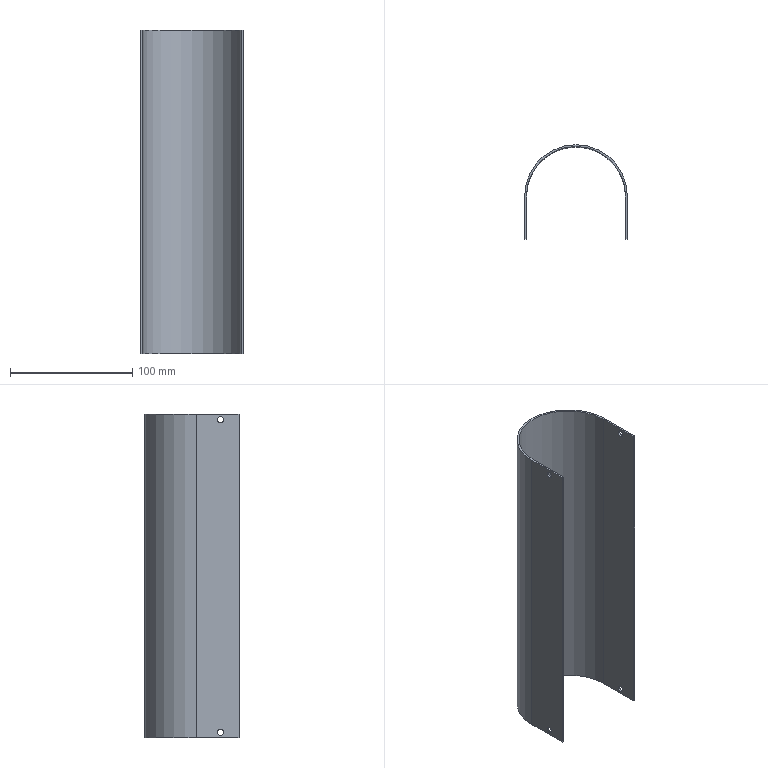Part | SolidWorks | features Extrusion 1, ICE 1 | 1 solid | 18 faces | box 84 x 77 x 265 mm | volume 79219 mm3 | cylinder 10 | plane 8 | commonest cylinder face diameters 5 x8 81 x1 84 x1
STEP:
#1=CARTESIAN_POINT('',(-20.582,12.5,4.5));
#2=VERTEX_POINT('',#1);
#3=CARTESIAN_POINT('',(-20.582,17.5,4.5));
#4=VERTEX_POINT('',#3);
#5=CARTESIAN_POINT('',(-20.582,15.,4.5));
#6=DIRECTION('',(1.,0.,0.));
#7=DIRECTION('',(0.,1.,0.));
#8=AXIS2_PLACEMENT_3D('',#5,#6,#7);
#9=CIRCLE('',#8,2.5);
#10=EDGE_CURVE('',#2,#4,#9,.T.);
#11=ORIENTED_EDGE('',*,*,#10,.F.);
#12=CARTESIAN_POINT('',(-19.082,12.5,4.5));
#13=VERTEX_POINT('',#12);
#14=CARTESIAN_POINT('',(-20.582,12.5,4.5));
#15=DIRECTION('',(1.,0.,0.));
#16=VECTOR('',#15,1000.);
#17=LINE('',#14,#16);
#18=EDGE_CURVE('',#2,#13,#17,.T.);
#19=ORIENTED_EDGE('',*,*,#18,.T.);
#20=CARTESIAN_POINT('',(-19.082,17.5,4.5));
#21=VERTEX_POINT('',#20);
#22=CARTESIAN_POINT('',(-19.082,15.,4.5));
#23=DIRECTION('',(-1.,0.,0.));
#24=DIRECTION('',(0.,-1.,0.));
#25=AXIS2_PLACEMENT_3D('',#22,#23,#24);
#26=CIRCLE('',#25,2.5);
#27=EDGE_CURVE('',#21,#13,#26,.T.);
#28=ORIENTED_EDGE('',*,*,#27,.F.);
#29=CARTESIAN_POINT('',(-20.582,17.5,4.5));
#30=DIRECTION('',(1.,0.,0.));
#31=VECTOR('',#30,1000.);
#32=LINE('',#29,#31);
#33=EDGE_CURVE('',#4,#21,#32,.T.);
#34=ORIENTED_EDGE('',*,*,#33,.F.);
#35=EDGE_LOOP('',(#11,#19,#28,#34));
#36=FACE_OUTER_BOUND('',#35,.T.);
#37=CARTESIAN_POINT('',(-20.582,15.,4.5));
#38=DIRECTION('',(1.,0.,0.));
#39=DIRECTION('',(0.,1.,0.));
#40=AXIS2_PLACEMENT_3D('',#37,#38,#39);
#41=CYLINDRICAL_SURFACE('',#40,2.5);
#42=ADVANCED_FACE('',(#36),#41,.F.);
#43=CARTESIAN_POINT('',(61.918,12.5,4.5));
#44=VERTEX_POINT('',#43);
#45=CARTESIAN_POINT('',(61.918,17.5,4.5));
#46=VERTEX_POINT('',#45);
#47=CARTESIAN_POINT('',(61.918,15.,4.5));
#48=DIRECTION('',(1.,0.,0.));
#49=DIRECTION('',(0.,0.,-1.));
#50=AXIS2_PLACEMENT_3D('',#47,#48,#49);
#51=CIRCLE('',#50,2.5);
#52=EDGE_CURVE('',#44,#46,#51,.T.);
#53=ORIENTED_EDGE('',*,*,#52,.F.);
#54=CARTESIAN_POINT('',(63.418,12.5,4.5));
#55=VERTEX_POINT('',#54);
#56=CARTESIAN_POINT('',(-20.582,12.5,4.5));
#57=DIRECTION('',(1.,0.,0.));
#58=VECTOR('',#57,1000.);
#59=LINE('',#56,#58);
#60=EDGE_CURVE('',#44,#55,#59,.T.);
#61=ORIENTED_EDGE('',*,*,#60,.T.);
#62=CARTESIAN_POINT('',(63.418,17.5,4.5));
#63=VERTEX_POINT('',#62);
#64=CARTESIAN_POINT('',(63.418,15.,4.5));
#65=DIRECTION('',(1.,0.,0.));
#66=DIRECTION('',(0.,1.,0.));
#67=AXIS2_PLACEMENT_3D('',#64,#65,#66);
#68=CIRCLE('',#67,2.5);
#69=EDGE_CURVE('',#55,#63,#68,.T.);
#70=ORIENTED_EDGE('',*,*,#69,.T.);
#71=CARTESIAN_POINT('',(-20.582,17.5,4.5));
#72=DIRECTION('',(1.,0.,0.));
#73=VECTOR('',#72,1000.);
#74=LINE('',#71,#73);
#75=EDGE_CURVE('',#46,#63,#74,.T.);
#76=ORIENTED_EDGE('',*,*,#75,.F.);
#77=EDGE_LOOP('',(#53,#61,#70,#76));
#78=FACE_OUTER_BOUND('',#77,.T.);
#79=CARTESIAN_POINT('',(-20.582,15.,4.5));
#80=DIRECTION('',(1.,0.,0.));
#81=DIRECTION('',(0.,1.,0.));
#82=AXIS2_PLACEMENT_3D('',#79,#80,#81);
#83=CYLINDRICAL_SURFACE('',#82,2.5);
#84=ADVANCED_FACE('',(#78),#83,.F.);
#85=CARTESIAN_POINT('',(-20.582,12.5,260.5));
#86=VERTEX_POINT('',#85);
#87=CARTESIAN_POINT('',(-20.582,17.5,260.5));
#88=VERTEX_POINT('',#87);
#89=CARTESIAN_POINT('',(-20.582,15.,260.5));
#90=DIRECTION('',(1.,0.,0.));
#91=DIRECTION('',(0.,1.,0.));
#92=AXIS2_PLACEMENT_3D('',#89,#90,#91);
#93=CIRCLE('',#92,2.5);
#94=EDGE_CURVE('',#86,#88,#93,.T.);
#95=ORIENTED_EDGE('',*,*,#94,.F.);
#96=CARTESIAN_POINT('',(-19.082,12.5,260.5));
#97=VERTEX_POINT('',#96);
#98=CARTESIAN_POINT('',(-20.582,12.5,260.5));
#99=DIRECTION('',(1.,0.,0.));
#100=VECTOR('',#99,1000.);
#101=LINE('',#98,#100);
#102=EDGE_CURVE('',#86,#97,#101,.T.);
#103=ORIENTED_EDGE('',*,*,#102,.T.);
#104=CARTESIAN_POINT('',(-19.082,17.5,260.5));
#105=VERTEX_POINT('',#104);
#106=CARTESIAN_POINT('',(-19.082,15.,260.5));
#107=DIRECTION('',(-1.,0.,0.));
#108=DIRECTION('',(0.,-1.,0.));
#109=AXIS2_PLACEMENT_3D('',#106,#107,#108);
#110=CIRCLE('',#109,2.5);
#111=EDGE_CURVE('',#105,#97,#110,.T.);
#112=ORIENTED_EDGE('',*,*,#111,.F.);
#113=CARTESIAN_POINT('',(-20.582,17.5,260.5));
#114=DIRECTION('',(1.,0.,0.));
#115=VECTOR('',#114,1000.);
#116=LINE('',#113,#115);
#117=EDGE_CURVE('',#88,#105,#116,.T.);
#118=ORIENTED_EDGE('',*,*,#117,.F.);
#119=EDGE_LOOP('',(#95,#103,#112,#118));
#120=FACE_OUTER_BOUND('',#119,.T.);
#121=CARTESIAN_POINT('',(-20.582,15.,260.5));
#122=DIRECTION('',(1.,0.,0.));
#123=DIRECTION('',(0.,1.,0.));
#124=AXIS2_PLACEMENT_3D('',#121,#122,#123);
#125=CYLINDRICAL_SURFACE('',#124,2.5);
#126=ADVANCED_FACE('',(#120),#125,.F.);
#127=CARTESIAN_POINT('',(61.918,12.5,260.5));
#128=VERTEX_POINT('',#127);
#129=CARTESIAN_POINT('',(61.918,17.5,260.5));
#130=VERTEX_POINT('',#129);
#131=CARTESIAN_POINT('',(61.918,15.,260.5));
#132=DIRECTION('',(1.,0.,0.));
#133=DIRECTION('',(0.,0.,-1.));
#134=AXIS2_PLACEMENT_3D('',#131,#132,#133);
#135=CIRCLE('',#134,2.5);
#136=EDGE_CURVE('',#128,#130,#135,.T.);
#137=ORIENTED_EDGE('',*,*,#136,.F.);
#138=CARTESIAN_POINT('',(63.418,12.5,260.5));
#139=VERTEX_POINT('',#138);
#140=CARTESIAN_POINT('',(-20.582,12.5,260.5));
#141=DIRECTION('',(1.,0.,0.));
#142=VECTOR('',#141,1000.);
#143=LINE('',#140,#142);
#144=EDGE_CURVE('',#128,#139,#143,.T.);
#145=ORIENTED_EDGE('',*,*,#144,.T.);
#146=CARTESIAN_POINT('',(63.418,17.5,260.5));
#147=VERTEX_POINT('',#146);
#148=CARTESIAN_POINT('',(63.418,15.,260.5));
#149=DIRECTION('',(1.,0.,0.));
#150=DIRECTION('',(0.,1.,0.));
#151=AXIS2_PLACEMENT_3D('',#148,#149,#150);
#152=CIRCLE('',#151,2.5);
#153=EDGE_CURVE('',#139,#147,#152,.T.);
#154=ORIENTED_EDGE('',*,*,#153,.T.);
#155=CARTESIAN_POINT('',(-20.582,17.5,260.5));
#156=DIRECTION('',(1.,0.,0.));
#157=VECTOR('',#156,1000.);
#158=LINE('',#155,#157);
#159=EDGE_CURVE('',#130,#147,#158,.T.);
#160=ORIENTED_EDGE('',*,*,#159,.F.);
#161=EDGE_LOOP('',(#137,#145,#154,#160));
#162=FACE_OUTER_BOUND('',#161,.T.);
#163=CARTESIAN_POINT('',(-20.582,15.,260.5));
#164=DIRECTION('',(1.,0.,0.));
#165=DIRECTION('',(0.,1.,0.));
#166=AXIS2_PLACEMENT_3D('',#163,#164,#165);
#167=CYLINDRICAL_SURFACE('',#166,2.5);
#168=ADVANCED_FACE('',(#162),#167,.F.);
#169=CARTESIAN_POINT('',(63.418,35.,0.));
#170=VERTEX_POINT('',#169);
#171=CARTESIAN_POINT('',(-20.582,35.,0.));
#172=VERTEX_POINT('',#171);
#173=CARTESIAN_POINT('',(21.418,35.,0.));
#174=DIRECTION('',(0.,0.,1.));
#175=DIRECTION('',(1.,0.,0.));
#176=AXIS2_PLACEMENT_3D('',#173,#174,#175);
#177=CIRCLE('',#176,42.);
#178=EDGE_CURVE('',#170,#172,#177,.T.);
#179=ORIENTED_EDGE('',*,*,#178,.T.);
#180=CARTESIAN_POINT('',(-20.582,35.,265.));
#181=VERTEX_POINT('',#180);
#182=CARTESIAN_POINT('',(-20.582,35.,265.));
#183=DIRECTION('',(0.,0.,-1.));
#184=VECTOR('',#183,1000.);
#185=LINE('',#182,#184);
#186=EDGE_CURVE('',#181,#172,#185,.T.);
#187=ORIENTED_EDGE('',*,*,#186,.F.);
#188=CARTESIAN_POINT('',(63.418,35.,265.));
#189=VERTEX_POINT('',#188);
#190=CARTESIAN_POINT('',(21.418,35.,265.));
#191=DIRECTION('',(0.,0.,1.));
#192=DIRECTION('',(1.,0.,0.));
#193=AXIS2_PLACEMENT_3D('',#190,#191,#192);
#194=CIRCLE('',#193,42.);
#195=EDGE_CURVE('',#189,#181,#194,.T.);
#196=ORIENTED_EDGE('',*,*,#195,.F.);
#197=CARTESIAN_POINT('',(63.418,35.,265.));
#198=DIRECTION('',(0.,0.,-1.));
#199=VECTOR('',#198,1000.);
#200=LINE('',#197,#199);
#201=EDGE_CURVE('',#189,#170,#200,.T.);
#202=ORIENTED_EDGE('',*,*,#201,.T.);
#203=EDGE_LOOP('',(#179,#187,#196,#202));
#204=FACE_OUTER_BOUND('',#203,.T.);
#205=CARTESIAN_POINT('',(21.418,35.,265.));
#206=DIRECTION('',(0.,0.,-1.));
#207=DIRECTION('',(-1.,0.,0.));
#208=AXIS2_PLACEMENT_3D('',#205,#206,#207);
#209=CYLINDRICAL_SURFACE('',#208,42.);
#210=ADVANCED_FACE('',(#204),#209,.T.);
#211=CARTESIAN_POINT('',(-20.582,15.,4.5));
#212=DIRECTION('',(1.,0.,0.));
#213=DIRECTION('',(0.,1.,0.));
#214=AXIS2_PLACEMENT_3D('',#211,#212,#213);
#215=CIRCLE('',#214,2.5);
#216=EDGE_CURVE('',#4,#2,#215,.T.);
#217=ORIENTED_EDGE('',*,*,#216,.T.);
#218=ORIENTED_EDGE('',*,*,#10,.T.);
#219=EDGE_LOOP('',(#217,#218));
#220=FACE_BOUND('',#219,.T.);
#221=CARTESIAN_POINT('',(-20.582,15.,260.5));
#222=DIRECTION('',(1.,0.,0.));
#223=DIRECTION('',(0.,1.,0.));
#224=AXIS2_PLACEMENT_3D('',#221,#222,#223);
#225=CIRCLE('',#224,2.5);
#226=EDGE_CURVE('',#88,#86,#225,.T.);
#227=ORIENTED_EDGE('',*,*,#226,.T.);
#228=ORIENTED_EDGE('',*,*,#94,.T.);
#229=EDGE_LOOP('',(#227,#228));
#230=FACE_BOUND('',#229,.T.);
#231=CARTESIAN_POINT('',(-20.582,0.,0.));
#232=VERTEX_POINT('',#231);
#233=CARTESIAN_POINT('',(-20.582,35.,0.));
#234=DIRECTION('',(0.,-1.,0.));
#235=VECTOR('',#234,1000.);
#236=LINE('',#233,#235);
#237=EDGE_CURVE('',#172,#232,#236,.T.);
#238=ORIENTED_EDGE('',*,*,#237,.T.);
#239=CARTESIAN_POINT('',(-20.582,0.,265.));
#240=VERTEX_POINT('',#239);
#241=CARTESIAN_POINT('',(-20.582,0.,265.));
#242=DIRECTION('',(0.,0.,-1.));
#243=VECTOR('',#242,1000.);
#244=LINE('',#241,#243);
#245=EDGE_CURVE('',#240,#232,#244,.T.);
#246=ORIENTED_EDGE('',*,*,#245,.F.);
#247=CARTESIAN_POINT('',(-20.582,35.,265.));
#248=DIRECTION('',(0.,-1.,0.));
#249=VECTOR('',#248,1000.);
#250=LINE('',#247,#249);
#251=EDGE_CURVE('',#181,#240,#250,.T.);
#252=ORIENTED_EDGE('',*,*,#251,.F.);
#253=ORIENTED_EDGE('',*,*,#186,.T.);
#254=EDGE_LOOP('',(#238,#246,#252,#253));
#255=FACE_OUTER_BOUND('',#254,.T.);
#256=CARTESIAN_POINT('',(-20.582,35.,265.));
#257=DIRECTION('',(1.,0.,0.));
#258=DIRECTION('',(0.,1.,0.));
#259=AXIS2_PLACEMENT_3D('',#256,#257,#258);
#260=PLANE('',#259);
#261=ADVANCED_FACE('',(#220,#230,#255),#260,.F.);
#262=CARTESIAN_POINT('',(-19.082,0.,0.));
#263=VERTEX_POINT('',#262);
#264=CARTESIAN_POINT('',(-20.582,0.,0.));
#265=DIRECTION('',(1.,0.,0.));
#266=VECTOR('',#265,1000.);
#267=LINE('',#264,#266);
#268=EDGE_CURVE('',#232,#263,#267,.T.);
#269=ORIENTED_EDGE('',*,*,#268,.T.);
#270=CARTESIAN_POINT('',(-19.082,0.,265.));
#271=VERTEX_POINT('',#270);
#272=CARTESIAN_POINT('',(-19.082,0.,265.));
#273=DIRECTION('',(0.,0.,-1.));
#274=VECTOR('',#273,1000.);
#275=LINE('',#272,#274);
#276=EDGE_CURVE('',#271,#263,#275,.T.);
#277=ORIENTED_EDGE('',*,*,#276,.F.);
#278=CARTESIAN_POINT('',(-20.582,0.,265.));
#279=DIRECTION('',(1.,0.,0.));
#280=VECTOR('',#279,1000.);
#281=LINE('',#278,#280);
#282=EDGE_CURVE('',#240,#271,#281,.T.);
#283=ORIENTED_EDGE('',*,*,#282,.F.);
#284=ORIENTED_EDGE('',*,*,#245,.T.);
#285=EDGE_LOOP('',(#269,#277,#283,#284));
#286=FACE_OUTER_BOUND('',#285,.T.);
#287=CARTESIAN_POINT('',(-20.582,0.,265.));
#288=DIRECTION('',(0.,1.,0.));
#289=DIRECTION('',(-1.,0.,0.));
#290=AXIS2_PLACEMENT_3D('',#287,#288,#289);
#291=PLANE('',#290);
#292=ADVANCED_FACE('',(#286),#291,.F.);
#293=ORIENTED_EDGE('',*,*,#27,.T.);
#294=CARTESIAN_POINT('',(-19.082,15.,4.5));
#295=DIRECTION('',(-1.,0.,0.));
#296=DIRECTION('',(0.,-1.,0.));
#297=AXIS2_PLACEMENT_3D('',#294,#295,#296);
#298=CIRCLE('',#297,2.5);
#299=EDGE_CURVE('',#13,#21,#298,.T.);
#300=ORIENTED_EDGE('',*,*,#299,.T.);
#301=EDGE_LOOP('',(#293,#300));
#302=FACE_BOUND('',#301,.T.);
#303=ORIENTED_EDGE('',*,*,#111,.T.);
#304=CARTESIAN_POINT('',(-19.082,15.,260.5));
#305=DIRECTION('',(-1.,0.,0.));
#306=DIRECTION('',(0.,-1.,0.));
#307=AXIS2_PLACEMENT_3D('',#304,#305,#306);
#308=CIRCLE('',#307,2.5);
#309=EDGE_CURVE('',#97,#105,#308,.T.);
#310=ORIENTED_EDGE('',*,*,#309,.T.);
#311=EDGE_LOOP('',(#303,#310));
#312=FACE_BOUND('',#311,.T.);
#313=CARTESIAN_POINT('',(-19.082,35.,0.));
#314=VERTEX_POINT('',#313);
#315=CARTESIAN_POINT('',(-19.082,35.,0.));
#316=DIRECTION('',(0.,1.,0.));
#317=VECTOR('',#316,1000.);
#318=LINE('',#315,#317);
#319=EDGE_CURVE('',#263,#314,#318,.T.);
#320=ORIENTED_EDGE('',*,*,#319,.T.);
#321=CARTESIAN_POINT('',(-19.082,35.,265.));
#322=VERTEX_POINT('',#321);
#323=CARTESIAN_POINT('',(-19.082,35.,265.));
#324=DIRECTION('',(0.,0.,-1.));
#325=VECTOR('',#324,1000.);
#326=LINE('',#323,#325);
#327=EDGE_CURVE('',#322,#314,#326,.T.);
#328=ORIENTED_EDGE('',*,*,#327,.F.);
#329=CARTESIAN_POINT('',(-19.082,35.,265.));
#330=DIRECTION('',(0.,1.,0.));
#331=VECTOR('',#330,1000.);
#332=LINE('',#329,#331);
#333=EDGE_CURVE('',#271,#322,#332,.T.);
#334=ORIENTED_EDGE('',*,*,#333,.F.);
#335=ORIENTED_EDGE('',*,*,#276,.T.);
#336=EDGE_LOOP('',(#320,#328,#334,#335));
#337=FACE_OUTER_BOUND('',#336,.T.);
#338=CARTESIAN_POINT('',(-19.082,35.,265.));
#339=DIRECTION('',(-1.,0.,0.));
#340=DIRECTION('',(0.,-1.,0.));
#341=AXIS2_PLACEMENT_3D('',#338,#339,#340);
#342=PLANE('',#341);
#343=ADVANCED_FACE('',(#302,#312,#337),#342,.F.);
#344=CARTESIAN_POINT('',(61.918,35.,0.));
#345=VERTEX_POINT('',#344);
#346=CARTESIAN_POINT('',(21.418,35.,0.));
#347=DIRECTION('',(0.,0.,-1.));
#348=DIRECTION('',(1.,0.,0.));
#349=AXIS2_PLACEMENT_3D('',#346,#347,#348);
#350=CIRCLE('',#349,40.5);
#351=EDGE_CURVE('',#314,#345,#350,.T.);
#352=ORIENTED_EDGE('',*,*,#351,.T.);
#353=CARTESIAN_POINT('',(61.918,35.,265.));
#354=VERTEX_POINT('',#353);
#355=CARTESIAN_POINT('',(61.918,35.,265.));
#356=DIRECTION('',(0.,0.,-1.));
#357=VECTOR('',#356,1000.);
#358=LINE('',#355,#357);
#359=EDGE_CURVE('',#354,#345,#358,.T.);
#360=ORIENTED_EDGE('',*,*,#359,.F.);
#361=CARTESIAN_POINT('',(21.418,35.,265.));
#362=DIRECTION('',(0.,0.,-1.));
#363=DIRECTION('',(1.,0.,0.));
#364=AXIS2_PLACEMENT_3D('',#361,#362,#363);
#365=CIRCLE('',#364,40.5);
#366=EDGE_CURVE('',#322,#354,#365,.T.);
#367=ORIENTED_EDGE('',*,*,#366,.F.);
#368=ORIENTED_EDGE('',*,*,#327,.T.);
#369=EDGE_LOOP('',(#352,#360,#367,#368));
#370=FACE_OUTER_BOUND('',#369,.T.);
#371=CARTESIAN_POINT('',(21.418,35.,265.));
#372=DIRECTION('',(0.,0.,-1.));
#373=DIRECTION('',(-1.,0.,0.));
#374=AXIS2_PLACEMENT_3D('',#371,#372,#373);
#375=CYLINDRICAL_SURFACE('',#374,40.5);
#376=ADVANCED_FACE('',(#370),#375,.F.);
#377=CARTESIAN_POINT('',(61.918,15.,4.5));
#378=DIRECTION('',(1.,0.,0.));
#379=DIRECTION('',(0.,0.,-1.));
#380=AXIS2_PLACEMENT_3D('',#377,#378,#379);
#381=CIRCLE('',#380,2.5);
#382=EDGE_CURVE('',#46,#44,#381,.T.);
#383=ORIENTED_EDGE('',*,*,#382,.T.);
#384=ORIENTED_EDGE('',*,*,#52,.T.);
#385=EDGE_LOOP('',(#383,#384));
#386=FACE_BOUND('',#385,.T.);
#387=CARTESIAN_POINT('',(61.918,15.,260.5));
#388=DIRECTION('',(1.,0.,0.));
#389=DIRECTION('',(0.,0.,-1.));
#390=AXIS2_PLACEMENT_3D('',#387,#388,#389);
#391=CIRCLE('',#390,2.5);
#392=EDGE_CURVE('',#130,#128,#391,.T.);
#393=ORIENTED_EDGE('',*,*,#392,.T.);
#394=ORIENTED_EDGE('',*,*,#136,.T.);
#395=EDGE_LOOP('',(#393,#394));
#396=FACE_BOUND('',#395,.T.);
#397=CARTESIAN_POINT('',(61.918,0.,0.));
#398=VERTEX_POINT('',#397);
#399=CARTESIAN_POINT('',(61.918,35.,0.));
#400=DIRECTION('',(0.,-1.,0.));
#401=VECTOR('',#400,1000.);
#402=LINE('',#399,#401);
#403=EDGE_CURVE('',#345,#398,#402,.T.);
#404=ORIENTED_EDGE('',*,*,#403,.T.);
#405=CARTESIAN_POINT('',(61.918,0.,265.));
#406=VERTEX_POINT('',#405);
#407=CARTESIAN_POINT('',(61.918,0.,265.));
#408=DIRECTION('',(0.,0.,-1.));
#409=VECTOR('',#408,1000.);
#410=LINE('',#407,#409);
#411=EDGE_CURVE('',#406,#398,#410,.T.);
#412=ORIENTED_EDGE('',*,*,#411,.F.);
#413=CARTESIAN_POINT('',(61.918,35.,265.));
#414=DIRECTION('',(0.,-1.,0.));
#415=VECTOR('',#414,1000.);
#416=LINE('',#413,#415);
#417=EDGE_CURVE('',#354,#406,#416,.T.);
#418=ORIENTED_EDGE('',*,*,#417,.F.);
#419=ORIENTED_EDGE('',*,*,#359,.T.);
#420=EDGE_LOOP('',(#404,#412,#418,#419));
#421=FACE_OUTER_BOUND('',#420,.T.);
#422=CARTESIAN_POINT('',(61.918,35.,265.));
#423=DIRECTION('',(1.,0.,0.));
#424=DIRECTION('',(0.,0.,-1.));
#425=AXIS2_PLACEMENT_3D('',#422,#423,#424);
#426=PLANE('',#425);
#427=ADVANCED_FACE('',(#386,#396,#421),#426,.F.);
#428=CARTESIAN_POINT('',(63.418,0.,0.));
#429=VERTEX_POINT('',#428);
#430=CARTESIAN_POINT('',(61.918,0.,0.));
#431=DIRECTION('',(1.,0.,0.));
#432=VECTOR('',#431,1000.);
#433=LINE('',#430,#432);
#434=EDGE_CURVE('',#398,#429,#433,.T.);
#435=ORIENTED_EDGE('',*,*,#434,.T.);
#436=CARTESIAN_POINT('',(63.418,0.,265.));
#437=VERTEX_POINT('',#436);
#438=CARTESIAN_POINT('',(63.418,0.,265.));
#439=DIRECTION('',(0.,0.,-1.));
#440=VECTOR('',#439,1000.);
#441=LINE('',#438,#440);
#442=EDGE_CURVE('',#437,#429,#441,.T.);
#443=ORIENTED_EDGE('',*,*,#442,.F.);
#444=CARTESIAN_POINT('',(61.918,0.,265.));
#445=DIRECTION('',(1.,0.,0.));
#446=VECTOR('',#445,1000.);
#447=LINE('',#444,#446);
#448=EDGE_CURVE('',#406,#437,#447,.T.);
#449=ORIENTED_EDGE('',*,*,#448,.F.);
#450=ORIENTED_EDGE('',*,*,#411,.T.);
#451=EDGE_LOOP('',(#435,#443,#449,#450));
#452=FACE_OUTER_BOUND('',#451,.T.);
#453=CARTESIAN_POINT('',(61.918,0.,265.));
#454=DIRECTION('',(0.,1.,0.));
#455=DIRECTION('',(-1.,0.,0.));
#456=AXIS2_PLACEMENT_3D('',#453,#454,#455);
#457=PLANE('',#456);
#458=ADVANCED_FACE('',(#452),#457,.F.);
#459=CARTESIAN_POINT('',(63.418,15.,4.5));
#460=DIRECTION('',(1.,0.,0.));
#461=DIRECTION('',(0.,1.,0.));
#462=AXIS2_PLACEMENT_3D('',#459,#460,#461);
#463=CIRCLE('',#462,2.5);
#464=EDGE_CURVE('',#63,#55,#463,.T.);
#465=ORIENTED_EDGE('',*,*,#464,.F.);
#466=ORIENTED_EDGE('',*,*,#69,.F.);
#467=EDGE_LOOP('',(#465,#466));
#468=FACE_BOUND('',#467,.T.);
#469=CARTESIAN_POINT('',(63.418,15.,260.5));
#470=DIRECTION('',(1.,0.,0.));
#471=DIRECTION('',(0.,1.,0.));
#472=AXIS2_PLACEMENT_3D('',#469,#470,#471);
#473=CIRCLE('',#472,2.5);
#474=EDGE_CURVE('',#147,#139,#473,.T.);
#475=ORIENTED_EDGE('',*,*,#474,.F.);
#476=ORIENTED_EDGE('',*,*,#153,.F.);
#477=EDGE_LOOP('',(#475,#476));
#478=FACE_BOUND('',#477,.T.);
#479=CARTESIAN_POINT('',(63.418,35.,0.));
#480=DIRECTION('',(0.,1.,0.));
#481=VECTOR('',#480,1000.);
#482=LINE('',#479,#481);
#483=EDGE_CURVE('',#429,#170,#482,.T.);
#484=ORIENTED_EDGE('',*,*,#483,.T.);
#485=ORIENTED_EDGE('',*,*,#201,.F.);
#486=CARTESIAN_POINT('',(63.418,35.,265.));
#487=DIRECTION('',(0.,1.,0.));
#488=VECTOR('',#487,1000.);
#489=LINE('',#486,#488);
#490=EDGE_CURVE('',#437,#189,#489,.T.);
#491=ORIENTED_EDGE('',*,*,#490,.F.);
#492=ORIENTED_EDGE('',*,*,#442,.T.);
#493=EDGE_LOOP('',(#484,#485,#491,#492));
#494=FACE_OUTER_BOUND('',#493,.T.);
#495=CARTESIAN_POINT('',(63.418,35.,265.));
#496=DIRECTION('',(-1.,0.,0.));
#497=DIRECTION('',(0.,-1.,0.));
#498=AXIS2_PLACEMENT_3D('',#495,#496,#497);
#499=PLANE('',#498);
#500=ADVANCED_FACE('',(#468,#478,#494),#499,.F.);
#501=ORIENTED_EDGE('',*,*,#195,.T.);
#502=ORIENTED_EDGE('',*,*,#251,.T.);
#503=ORIENTED_EDGE('',*,*,#282,.T.);
#504=ORIENTED_EDGE('',*,*,#333,.T.);
#505=ORIENTED_EDGE('',*,*,#366,.T.);
#506=ORIENTED_EDGE('',*,*,#417,.T.);
#507=ORIENTED_EDGE('',*,*,#448,.T.);
#508=ORIENTED_EDGE('',*,*,#490,.T.);
#509=EDGE_LOOP('',(#501,#502,#503,#504,#505,#506,#507,#508));
#510=FACE_OUTER_BOUND('',#509,.T.);
#511=CARTESIAN_POINT('',(21.418,35.,265.));
#512=DIRECTION('',(0.,0.,1.));
#513=DIRECTION('',(1.,0.,0.));
#514=AXIS2_PLACEMENT_3D('',#511,#512,#513);
#515=PLANE('',#514);
#516=ADVANCED_FACE('',(#510),#515,.T.);
#517=ORIENTED_EDGE('',*,*,#178,.F.);
#518=ORIENTED_EDGE('',*,*,#483,.F.);
#519=ORIENTED_EDGE('',*,*,#434,.F.);
#520=ORIENTED_EDGE('',*,*,#403,.F.);
#521=ORIENTED_EDGE('',*,*,#351,.F.);
#522=ORIENTED_EDGE('',*,*,#319,.F.);
#523=ORIENTED_EDGE('',*,*,#268,.F.);
#524=ORIENTED_EDGE('',*,*,#237,.F.);
#525=EDGE_LOOP('',(#517,#518,#519,#520,#521,#522,#523,#524));
#526=FACE_OUTER_BOUND('',#525,.T.);
#527=CARTESIAN_POINT('',(21.418,35.,0.));
#528=DIRECTION('',(0.,0.,1.));
#529=DIRECTION('',(1.,0.,0.));
#530=AXIS2_PLACEMENT_3D('',#527,#528,#529);
#531=PLANE('',#530);
#532=ADVANCED_FACE('',(#526),#531,.F.);
#533=ORIENTED_EDGE('',*,*,#144,.F.);
#534=ORIENTED_EDGE('',*,*,#392,.F.);
#535=ORIENTED_EDGE('',*,*,#159,.T.);
#536=ORIENTED_EDGE('',*,*,#474,.T.);
#537=EDGE_LOOP('',(#533,#534,#535,#536));
#538=FACE_OUTER_BOUND('',#537,.T.);
#539=CARTESIAN_POINT('',(-20.582,15.,260.5));
#540=DIRECTION('',(1.,0.,0.));
#541=DIRECTION('',(0.,1.,0.));
#542=AXIS2_PLACEMENT_3D('',#539,#540,#541);
#543=CYLINDRICAL_SURFACE('',#542,2.5);
#544=ADVANCED_FACE('',(#538),#543,.F.);
#545=ORIENTED_EDGE('',*,*,#102,.F.);
#546=ORIENTED_EDGE('',*,*,#226,.F.);
#547=ORIENTED_EDGE('',*,*,#117,.T.);
#548=ORIENTED_EDGE('',*,*,#309,.F.);
#549=EDGE_LOOP('',(#545,#546,#547,#548));
#550=FACE_OUTER_BOUND('',#549,.T.);
#551=CARTESIAN_POINT('',(-20.582,15.,260.5));
#552=DIRECTION('',(1.,0.,0.));
#553=DIRECTION('',(0.,1.,0.));
#554=AXIS2_PLACEMENT_3D('',#551,#552,#553);
#555=CYLINDRICAL_SURFACE('',#554,2.5);
#556=ADVANCED_FACE('',(#550),#555,.F.);
#557=ORIENTED_EDGE('',*,*,#60,.F.);
#558=ORIENTED_EDGE('',*,*,#382,.F.);
#559=ORIENTED_EDGE('',*,*,#75,.T.);
#560=ORIENTED_EDGE('',*,*,#464,.T.);
#561=EDGE_LOOP('',(#557,#558,#559,#560));
#562=FACE_OUTER_BOUND('',#561,.T.);
#563=CARTESIAN_POINT('',(-20.582,15.,4.5));
#564=DIRECTION('',(1.,0.,0.));
#565=DIRECTION('',(0.,1.,0.));
#566=AXIS2_PLACEMENT_3D('',#563,#564,#565);
#567=CYLINDRICAL_SURFACE('',#566,2.5);
#568=ADVANCED_FACE('',(#562),#567,.F.);
#569=ORIENTED_EDGE('',*,*,#18,.F.);
#570=ORIENTED_EDGE('',*,*,#216,.F.);
#571=ORIENTED_EDGE('',*,*,#33,.T.);
#572=ORIENTED_EDGE('',*,*,#299,.F.);
#573=EDGE_LOOP('',(#569,#570,#571,#572));
#574=FACE_OUTER_BOUND('',#573,.T.);
#575=CARTESIAN_POINT('',(-20.582,15.,4.5));
#576=DIRECTION('',(1.,0.,0.));
#577=DIRECTION('',(0.,1.,0.));
#578=AXIS2_PLACEMENT_3D('',#575,#576,#577);
#579=CYLINDRICAL_SURFACE('',#578,2.5);
#580=ADVANCED_FACE('',(#574),#579,.F.);
#581=CLOSED_SHELL('',(#42,#84,#126,#168,#210,#261,#292,#343,#376,#427,#458,#500,#516,#532,#544,#556,#568,#580));
#582=MANIFOLD_SOLID_BREP('',#581);
#583=CARTESIAN_POINT('',(0.,0.,0.));
#584=DIRECTION('',(0.,0.,1.));
#585=DIRECTION('',(1.,0.,0.));
#586=AXIS2_PLACEMENT_3D('',#583,#584,#585);
#587=(LENGTH_UNIT()NAMED_UNIT(*)SI_UNIT(.MILLI.,.METRE.));
#588=UNCERTAINTY_MEASURE_WITH_UNIT(LENGTH_MEASURE(0.00001),#587,'','');
#589=(NAMED_UNIT(*)PLANE_ANGLE_UNIT()SI_UNIT($,.RADIAN.));
#590=(NAMED_UNIT(*)SI_UNIT($,.STERADIAN.)SOLID_ANGLE_UNIT());
#591=(GEOMETRIC_REPRESENTATION_CONTEXT(3)GLOBAL_UNCERTAINTY_ASSIGNED_CONTEXT((#588))GLOBAL_UNIT_ASSIGNED_CONTEXT((#587,#589,#590))REPRESENTATION_CONTEXT('',''));
#592=ADVANCED_BREP_SHAPE_REPRESENTATION('',(#582,#586),#591);